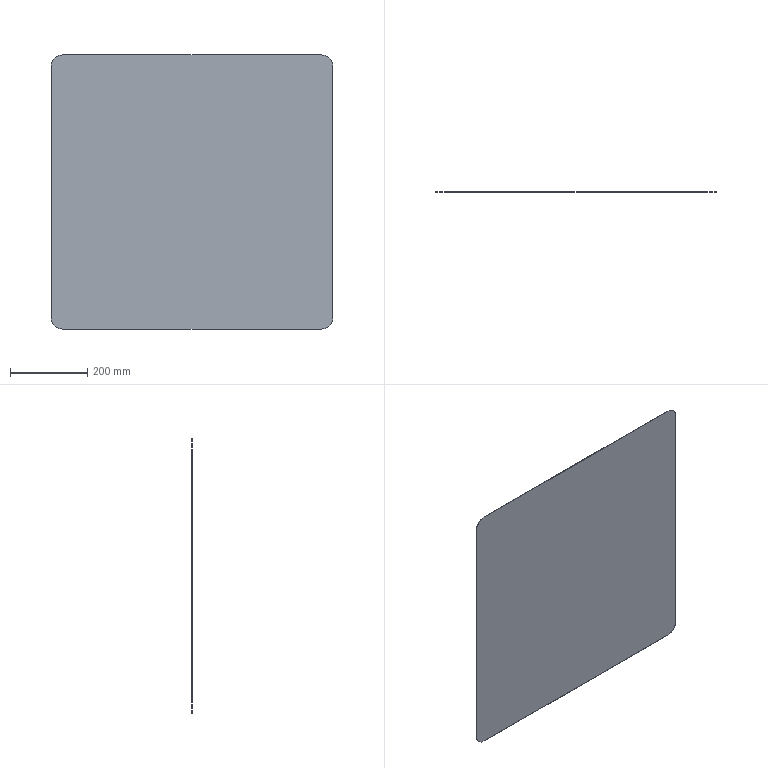Part | STEP file | 冲床-300配套压波_id518_x_t | 1 solid | 10 faces | box 730 x 1.2 x 710 mm | volume 621033 mm3 | plane 6 | cylinder 4 | commonest cylinder face diameters 60 x4
STEP:
#1=CARTESIAN_POINT('',(1175.,-280.,-75.));
#2=VERTEX_POINT('',#1);
#3=CARTESIAN_POINT('',(1175.,-280.,-725.));
#4=VERTEX_POINT('',#3);
#5=CARTESIAN_POINT('',(1175.,-280.,-755.));
#6=DIRECTION('',(0.,0.,-1.));
#7=VECTOR('',#6,1.);
#8=LINE('',#5,#7);
#9=EDGE_CURVE('',#2,#4,#8,.T.);
#10=ORIENTED_EDGE('',*,*,#9,.T.);
#11=CARTESIAN_POINT('',(1175.,-281.2,-725.));
#12=VERTEX_POINT('',#11);
#13=CARTESIAN_POINT('',(1175.,-281.2,-725.));
#14=DIRECTION('',(0.,-1.,0.));
#15=VECTOR('',#14,1.);
#16=LINE('',#13,#15);
#17=EDGE_CURVE('',#4,#12,#16,.T.);
#18=ORIENTED_EDGE('',*,*,#17,.T.);
#19=CARTESIAN_POINT('',(1175.,-281.2,-75.));
#20=VERTEX_POINT('',#19);
#21=CARTESIAN_POINT('',(1175.,-281.2,-755.));
#22=DIRECTION('',(0.,0.,-1.));
#23=VECTOR('',#22,1.);
#24=LINE('',#21,#23);
#25=EDGE_CURVE('',#20,#12,#24,.T.);
#26=ORIENTED_EDGE('',*,*,#25,.F.);
#27=CARTESIAN_POINT('',(1175.,-281.2,-75.));
#28=DIRECTION('',(0.,1.,0.));
#29=VECTOR('',#28,1.);
#30=LINE('',#27,#29);
#31=EDGE_CURVE('',#20,#2,#30,.T.);
#32=ORIENTED_EDGE('',*,*,#31,.T.);
#33=EDGE_LOOP('',(#10,#18,#26,#32));
#34=FACE_OUTER_BOUND('',#33,.T.);
#35=CARTESIAN_POINT('',(1175.,-281.2,-755.));
#36=DIRECTION('',(1.,0.,0.));
#37=DIRECTION('',(0.,0.,-1.));
#38=AXIS2_PLACEMENT_3D('',#35,#36,#37);
#39=PLANE('',#38);
#40=ADVANCED_FACE('',(#34),#39,.F.);
#41=CARTESIAN_POINT('',(1875.,-281.2,-45.));
#42=VERTEX_POINT('',#41);
#43=CARTESIAN_POINT('',(1205.,-281.2,-45.));
#44=VERTEX_POINT('',#43);
#45=CARTESIAN_POINT('',(1185.,-281.2,-45.));
#46=DIRECTION('',(-1.,0.,0.));
#47=VECTOR('',#46,1.);
#48=LINE('',#45,#47);
#49=EDGE_CURVE('',#42,#44,#48,.T.);
#50=ORIENTED_EDGE('',*,*,#49,.F.);
#51=CARTESIAN_POINT('',(1875.,-280.,-45.));
#52=VERTEX_POINT('',#51);
#53=CARTESIAN_POINT('',(1875.,-281.2,-45.));
#54=DIRECTION('',(0.,1.,0.));
#55=VECTOR('',#54,1.);
#56=LINE('',#53,#55);
#57=EDGE_CURVE('',#42,#52,#56,.T.);
#58=ORIENTED_EDGE('',*,*,#57,.T.);
#59=CARTESIAN_POINT('',(1205.,-280.,-45.));
#60=VERTEX_POINT('',#59);
#61=CARTESIAN_POINT('',(1185.,-280.,-45.));
#62=DIRECTION('',(-1.,0.,0.));
#63=VECTOR('',#62,1.);
#64=LINE('',#61,#63);
#65=EDGE_CURVE('',#52,#60,#64,.T.);
#66=ORIENTED_EDGE('',*,*,#65,.T.);
#67=CARTESIAN_POINT('',(1205.,-281.2,-45.));
#68=DIRECTION('',(0.,-1.,0.));
#69=VECTOR('',#68,1.);
#70=LINE('',#67,#69);
#71=EDGE_CURVE('',#60,#44,#70,.T.);
#72=ORIENTED_EDGE('',*,*,#71,.T.);
#73=EDGE_LOOP('',(#50,#58,#66,#72));
#74=FACE_OUTER_BOUND('',#73,.T.);
#75=CARTESIAN_POINT('',(1185.,-281.2,-45.));
#76=DIRECTION('',(0.,0.,-1.));
#77=DIRECTION('',(-1.,0.,0.));
#78=AXIS2_PLACEMENT_3D('',#75,#76,#77);
#79=PLANE('',#78);
#80=ADVANCED_FACE('',(#74),#79,.F.);
#81=CARTESIAN_POINT('',(1905.,-280.,-725.));
#82=VERTEX_POINT('',#81);
#83=CARTESIAN_POINT('',(1905.,-280.,-75.));
#84=VERTEX_POINT('',#83);
#85=CARTESIAN_POINT('',(1905.,-280.,-45.));
#86=DIRECTION('',(0.,0.,1.));
#87=VECTOR('',#86,1.);
#88=LINE('',#85,#87);
#89=EDGE_CURVE('',#82,#84,#88,.T.);
#90=ORIENTED_EDGE('',*,*,#89,.T.);
#91=CARTESIAN_POINT('',(1905.,-281.2,-75.));
#92=VERTEX_POINT('',#91);
#93=CARTESIAN_POINT('',(1905.,-281.2,-75.));
#94=DIRECTION('',(0.,-1.,0.));
#95=VECTOR('',#94,1.);
#96=LINE('',#93,#95);
#97=EDGE_CURVE('',#84,#92,#96,.T.);
#98=ORIENTED_EDGE('',*,*,#97,.T.);
#99=CARTESIAN_POINT('',(1905.,-281.2,-725.));
#100=VERTEX_POINT('',#99);
#101=CARTESIAN_POINT('',(1905.,-281.2,-45.));
#102=DIRECTION('',(0.,0.,1.));
#103=VECTOR('',#102,1.);
#104=LINE('',#101,#103);
#105=EDGE_CURVE('',#100,#92,#104,.T.);
#106=ORIENTED_EDGE('',*,*,#105,.F.);
#107=CARTESIAN_POINT('',(1905.,-281.2,-725.));
#108=DIRECTION('',(0.,1.,0.));
#109=VECTOR('',#108,1.);
#110=LINE('',#107,#109);
#111=EDGE_CURVE('',#100,#82,#110,.T.);
#112=ORIENTED_EDGE('',*,*,#111,.T.);
#113=EDGE_LOOP('',(#90,#98,#106,#112));
#114=FACE_OUTER_BOUND('',#113,.T.);
#115=CARTESIAN_POINT('',(1905.,-281.2,-45.));
#116=DIRECTION('',(-1.,0.,0.));
#117=DIRECTION('',(0.,0.,1.));
#118=AXIS2_PLACEMENT_3D('',#115,#116,#117);
#119=PLANE('',#118);
#120=ADVANCED_FACE('',(#114),#119,.F.);
#121=CARTESIAN_POINT('',(1205.,-280.,-755.));
#122=VERTEX_POINT('',#121);
#123=CARTESIAN_POINT('',(1875.,-280.,-755.));
#124=VERTEX_POINT('',#123);
#125=CARTESIAN_POINT('',(1895.,-280.,-755.));
#126=DIRECTION('',(1.,0.,0.));
#127=VECTOR('',#126,1.);
#128=LINE('',#125,#127);
#129=EDGE_CURVE('',#122,#124,#128,.T.);
#130=ORIENTED_EDGE('',*,*,#129,.T.);
#131=CARTESIAN_POINT('',(1875.,-281.2,-755.));
#132=VERTEX_POINT('',#131);
#133=CARTESIAN_POINT('',(1875.,-281.2,-755.));
#134=DIRECTION('',(0.,-1.,0.));
#135=VECTOR('',#134,1.);
#136=LINE('',#133,#135);
#137=EDGE_CURVE('',#124,#132,#136,.T.);
#138=ORIENTED_EDGE('',*,*,#137,.T.);
#139=CARTESIAN_POINT('',(1205.,-281.2,-755.));
#140=VERTEX_POINT('',#139);
#141=CARTESIAN_POINT('',(1895.,-281.2,-755.));
#142=DIRECTION('',(1.,0.,0.));
#143=VECTOR('',#142,1.);
#144=LINE('',#141,#143);
#145=EDGE_CURVE('',#140,#132,#144,.T.);
#146=ORIENTED_EDGE('',*,*,#145,.F.);
#147=CARTESIAN_POINT('',(1205.,-281.2,-755.));
#148=DIRECTION('',(0.,1.,0.));
#149=VECTOR('',#148,1.);
#150=LINE('',#147,#149);
#151=EDGE_CURVE('',#140,#122,#150,.T.);
#152=ORIENTED_EDGE('',*,*,#151,.T.);
#153=EDGE_LOOP('',(#130,#138,#146,#152));
#154=FACE_OUTER_BOUND('',#153,.T.);
#155=CARTESIAN_POINT('',(1895.,-281.2,-755.));
#156=DIRECTION('',(0.,0.,1.));
#157=DIRECTION('',(1.,0.,0.));
#158=AXIS2_PLACEMENT_3D('',#155,#156,#157);
#159=PLANE('',#158);
#160=ADVANCED_FACE('',(#154),#159,.F.);
#161=ORIENTED_EDGE('',*,*,#105,.T.);
#162=CARTESIAN_POINT('',(1875.,-281.2,-75.));
#163=DIRECTION('',(0.,-1.,0.));
#164=DIRECTION('',(1.,0.,0.));
#165=AXIS2_PLACEMENT_3D('',#162,#163,#164);
#166=CIRCLE('',#165,30.);
#167=EDGE_CURVE('',#92,#42,#166,.T.);
#168=ORIENTED_EDGE('',*,*,#167,.T.);
#169=ORIENTED_EDGE('',*,*,#49,.T.);
#170=CARTESIAN_POINT('',(1205.,-281.2,-75.));
#171=DIRECTION('',(0.,-1.,0.));
#172=DIRECTION('',(1.,0.,0.));
#173=AXIS2_PLACEMENT_3D('',#170,#171,#172);
#174=CIRCLE('',#173,30.);
#175=EDGE_CURVE('',#44,#20,#174,.T.);
#176=ORIENTED_EDGE('',*,*,#175,.T.);
#177=ORIENTED_EDGE('',*,*,#25,.T.);
#178=CARTESIAN_POINT('',(1205.,-281.2,-725.));
#179=DIRECTION('',(0.,-1.,0.));
#180=DIRECTION('',(1.,0.,0.));
#181=AXIS2_PLACEMENT_3D('',#178,#179,#180);
#182=CIRCLE('',#181,30.);
#183=EDGE_CURVE('',#12,#140,#182,.T.);
#184=ORIENTED_EDGE('',*,*,#183,.T.);
#185=ORIENTED_EDGE('',*,*,#145,.T.);
#186=CARTESIAN_POINT('',(1875.,-281.2,-725.));
#187=DIRECTION('',(0.,-1.,0.));
#188=DIRECTION('',(1.,0.,0.));
#189=AXIS2_PLACEMENT_3D('',#186,#187,#188);
#190=CIRCLE('',#189,30.);
#191=EDGE_CURVE('',#132,#100,#190,.T.);
#192=ORIENTED_EDGE('',*,*,#191,.T.);
#193=EDGE_LOOP('',(#161,#168,#169,#176,#177,#184,#185,#192));
#194=FACE_OUTER_BOUND('',#193,.T.);
#195=CARTESIAN_POINT('',(0.,-281.2,10.));
#196=DIRECTION('',(0.,-1.,0.));
#197=DIRECTION('',(0.,0.,1.));
#198=AXIS2_PLACEMENT_3D('',#195,#196,#197);
#199=PLANE('',#198);
#200=ADVANCED_FACE('',(#194),#199,.T.);
#201=ORIENTED_EDGE('',*,*,#65,.F.);
#202=CARTESIAN_POINT('',(1875.,-280.,-75.));
#203=DIRECTION('',(0.,1.,0.));
#204=DIRECTION('',(1.,0.,0.));
#205=AXIS2_PLACEMENT_3D('',#202,#203,#204);
#206=CIRCLE('',#205,30.);
#207=EDGE_CURVE('',#52,#84,#206,.T.);
#208=ORIENTED_EDGE('',*,*,#207,.T.);
#209=ORIENTED_EDGE('',*,*,#89,.F.);
#210=CARTESIAN_POINT('',(1875.,-280.,-725.));
#211=DIRECTION('',(0.,1.,0.));
#212=DIRECTION('',(1.,0.,0.));
#213=AXIS2_PLACEMENT_3D('',#210,#211,#212);
#214=CIRCLE('',#213,30.);
#215=EDGE_CURVE('',#82,#124,#214,.T.);
#216=ORIENTED_EDGE('',*,*,#215,.T.);
#217=ORIENTED_EDGE('',*,*,#129,.F.);
#218=CARTESIAN_POINT('',(1205.,-280.,-725.));
#219=DIRECTION('',(0.,1.,0.));
#220=DIRECTION('',(1.,0.,0.));
#221=AXIS2_PLACEMENT_3D('',#218,#219,#220);
#222=CIRCLE('',#221,30.);
#223=EDGE_CURVE('',#122,#4,#222,.T.);
#224=ORIENTED_EDGE('',*,*,#223,.T.);
#225=ORIENTED_EDGE('',*,*,#9,.F.);
#226=CARTESIAN_POINT('',(1205.,-280.,-75.));
#227=DIRECTION('',(0.,1.,0.));
#228=DIRECTION('',(1.,0.,0.));
#229=AXIS2_PLACEMENT_3D('',#226,#227,#228);
#230=CIRCLE('',#229,30.);
#231=EDGE_CURVE('',#2,#60,#230,.T.);
#232=ORIENTED_EDGE('',*,*,#231,.T.);
#233=EDGE_LOOP('',(#201,#208,#209,#216,#217,#224,#225,#232));
#234=FACE_OUTER_BOUND('',#233,.T.);
#235=CARTESIAN_POINT('',(0.,-280.,10.));
#236=DIRECTION('',(0.,-1.,0.));
#237=DIRECTION('',(0.,0.,1.));
#238=AXIS2_PLACEMENT_3D('',#235,#236,#237);
#239=PLANE('',#238);
#240=ADVANCED_FACE('',(#234),#239,.F.);
#241=ORIENTED_EDGE('',*,*,#207,.F.);
#242=ORIENTED_EDGE('',*,*,#57,.F.);
#243=ORIENTED_EDGE('',*,*,#167,.F.);
#244=ORIENTED_EDGE('',*,*,#97,.F.);
#245=EDGE_LOOP('',(#241,#242,#243,#244));
#246=FACE_OUTER_BOUND('',#245,.T.);
#247=CARTESIAN_POINT('',(1875.,-281.2,-75.));
#248=DIRECTION('',(0.,-1.,0.));
#249=DIRECTION('',(1.,0.,0.));
#250=AXIS2_PLACEMENT_3D('',#247,#248,#249);
#251=CYLINDRICAL_SURFACE('',#250,30.);
#252=ADVANCED_FACE('',(#246),#251,.T.);
#253=ORIENTED_EDGE('',*,*,#215,.F.);
#254=ORIENTED_EDGE('',*,*,#111,.F.);
#255=ORIENTED_EDGE('',*,*,#191,.F.);
#256=ORIENTED_EDGE('',*,*,#137,.F.);
#257=EDGE_LOOP('',(#253,#254,#255,#256));
#258=FACE_OUTER_BOUND('',#257,.T.);
#259=CARTESIAN_POINT('',(1875.,-281.2,-725.));
#260=DIRECTION('',(0.,-1.,0.));
#261=DIRECTION('',(1.,0.,0.));
#262=AXIS2_PLACEMENT_3D('',#259,#260,#261);
#263=CYLINDRICAL_SURFACE('',#262,30.);
#264=ADVANCED_FACE('',(#258),#263,.T.);
#265=ORIENTED_EDGE('',*,*,#223,.F.);
#266=ORIENTED_EDGE('',*,*,#151,.F.);
#267=ORIENTED_EDGE('',*,*,#183,.F.);
#268=ORIENTED_EDGE('',*,*,#17,.F.);
#269=EDGE_LOOP('',(#265,#266,#267,#268));
#270=FACE_OUTER_BOUND('',#269,.T.);
#271=CARTESIAN_POINT('',(1205.,-281.2,-725.));
#272=DIRECTION('',(0.,-1.,0.));
#273=DIRECTION('',(1.,0.,0.));
#274=AXIS2_PLACEMENT_3D('',#271,#272,#273);
#275=CYLINDRICAL_SURFACE('',#274,30.);
#276=ADVANCED_FACE('',(#270),#275,.T.);
#277=ORIENTED_EDGE('',*,*,#231,.F.);
#278=ORIENTED_EDGE('',*,*,#31,.F.);
#279=ORIENTED_EDGE('',*,*,#175,.F.);
#280=ORIENTED_EDGE('',*,*,#71,.F.);
#281=EDGE_LOOP('',(#277,#278,#279,#280));
#282=FACE_OUTER_BOUND('',#281,.T.);
#283=CARTESIAN_POINT('',(1205.,-281.2,-75.));
#284=DIRECTION('',(0.,-1.,0.));
#285=DIRECTION('',(1.,0.,0.));
#286=AXIS2_PLACEMENT_3D('',#283,#284,#285);
#287=CYLINDRICAL_SURFACE('',#286,30.);
#288=ADVANCED_FACE('',(#282),#287,.T.);
#289=CLOSED_SHELL('',(#40,#80,#120,#160,#200,#240,#252,#264,#276,#288));
#290=MANIFOLD_SOLID_BREP('',#289);
#291=(LENGTH_UNIT()NAMED_UNIT(*)SI_UNIT(.MILLI.,.METRE.));
#292=UNCERTAINTY_MEASURE_WITH_UNIT(LENGTH_MEASURE(0.00002),#291,'','');
#293=(NAMED_UNIT(*)PLANE_ANGLE_UNIT()SI_UNIT($,.RADIAN.));
#294=PLANE_ANGLE_MEASURE_WITH_UNIT(PLANE_ANGLE_MEASURE(0.01745),#293);
#295=DIMENSIONAL_EXPONENTS(0.,0.,0.,0.,0.,0.,0.);
#296=(CONVERSION_BASED_UNIT('DEGREE',#294)NAMED_UNIT(#295)PLANE_ANGLE_UNIT());
#297=(NAMED_UNIT(*)SI_UNIT($,.STERADIAN.)SOLID_ANGLE_UNIT());
#298=(GEOMETRIC_REPRESENTATION_CONTEXT(3)GLOBAL_UNCERTAINTY_ASSIGNED_CONTEXT((#292))GLOBAL_UNIT_ASSIGNED_CONTEXT((#291,#296,#297))REPRESENTATION_CONTEXT('',''));
#299=ADVANCED_BREP_SHAPE_REPRESENTATION('',(#290),#298);